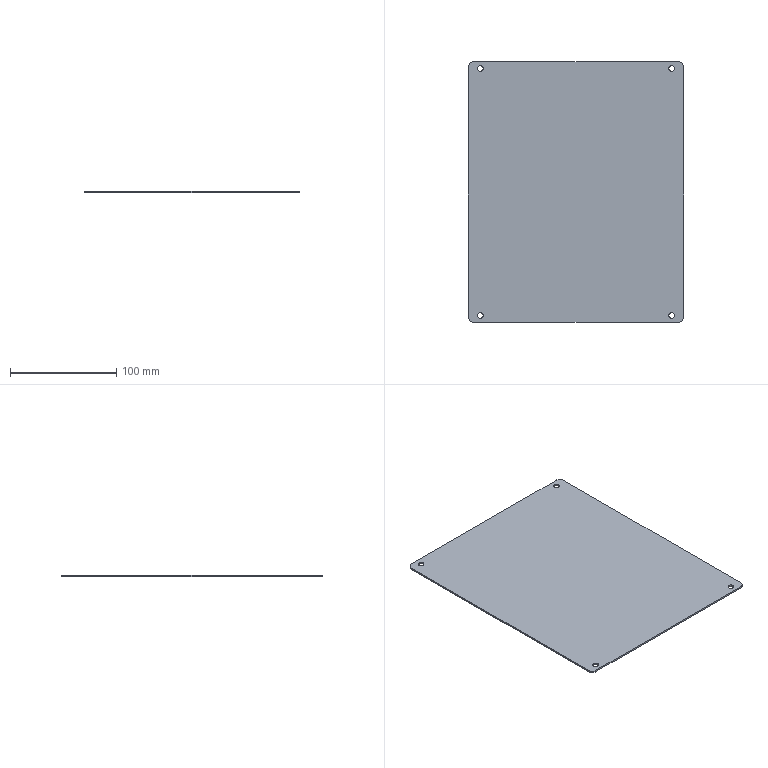Part | NX | features BREP 1 | 1 solid | 14 faces | box 202 x 245 x 1.5 mm | volume 74060 mm3 | cylinder 8 | plane 6 | commonest cylinder face diameters 5.5 x4 10 x4
STEP:
#1=CARTESIAN_POINT('',(-92.75,116.,0.));
#2=VERTEX_POINT('',#1);
#3=CARTESIAN_POINT('',(-90.,116.,0.));
#4=DIRECTION('',(0.,0.,1.));
#5=DIRECTION('',(-1.,0.,0.));
#6=AXIS2_PLACEMENT_3D('',#3,#4,#5);
#7=CIRCLE('',#6,2.75);
#8=EDGE_CURVE('',#2,#2,#7,.T.);
#9=ORIENTED_EDGE('',*,*,#8,.T.);
#10=EDGE_LOOP('',(#9));
#11=FACE_BOUND('',#10,.T.);
#12=CARTESIAN_POINT('',(-92.75,116.,-1.5));
#13=VERTEX_POINT('',#12);
#14=CARTESIAN_POINT('',(-90.,116.,-1.5));
#15=DIRECTION('',(0.,0.,-1.));
#16=DIRECTION('',(-1.,0.,0.));
#17=AXIS2_PLACEMENT_3D('',#14,#15,#16);
#18=CIRCLE('',#17,2.75);
#19=EDGE_CURVE('',#13,#13,#18,.T.);
#20=ORIENTED_EDGE('',*,*,#19,.T.);
#21=EDGE_LOOP('',(#20));
#22=FACE_BOUND('',#21,.T.);
#23=CARTESIAN_POINT('',(-90.,116.,-10.));
#24=DIRECTION('',(0.,0.,1.));
#25=DIRECTION('',(1.,0.,0.));
#26=AXIS2_PLACEMENT_3D('',#23,#24,#25);
#27=CYLINDRICAL_SURFACE('',#26,2.75);
#28=ADVANCED_FACE('',(#11,#22),#27,.F.);
#29=CARTESIAN_POINT('',(87.25,116.,0.));
#30=VERTEX_POINT('',#29);
#31=CARTESIAN_POINT('',(90.,116.,0.));
#32=DIRECTION('',(0.,0.,1.));
#33=DIRECTION('',(-1.,0.,0.));
#34=AXIS2_PLACEMENT_3D('',#31,#32,#33);
#35=CIRCLE('',#34,2.75);
#36=EDGE_CURVE('',#30,#30,#35,.T.);
#37=ORIENTED_EDGE('',*,*,#36,.T.);
#38=EDGE_LOOP('',(#37));
#39=FACE_BOUND('',#38,.T.);
#40=CARTESIAN_POINT('',(87.25,116.,-1.5));
#41=VERTEX_POINT('',#40);
#42=CARTESIAN_POINT('',(90.,116.,-1.5));
#43=DIRECTION('',(0.,0.,-1.));
#44=DIRECTION('',(-1.,0.,0.));
#45=AXIS2_PLACEMENT_3D('',#42,#43,#44);
#46=CIRCLE('',#45,2.75);
#47=EDGE_CURVE('',#41,#41,#46,.T.);
#48=ORIENTED_EDGE('',*,*,#47,.T.);
#49=EDGE_LOOP('',(#48));
#50=FACE_BOUND('',#49,.T.);
#51=CARTESIAN_POINT('',(90.,116.,-10.));
#52=DIRECTION('',(0.,0.,1.));
#53=DIRECTION('',(1.,0.,0.));
#54=AXIS2_PLACEMENT_3D('',#51,#52,#53);
#55=CYLINDRICAL_SURFACE('',#54,2.75);
#56=ADVANCED_FACE('',(#39,#50),#55,.F.);
#57=CARTESIAN_POINT('',(92.75,-116.,0.));
#58=VERTEX_POINT('',#57);
#59=CARTESIAN_POINT('',(90.,-116.,0.));
#60=DIRECTION('',(0.,0.,1.));
#61=DIRECTION('',(1.,0.,0.));
#62=AXIS2_PLACEMENT_3D('',#59,#60,#61);
#63=CIRCLE('',#62,2.75);
#64=EDGE_CURVE('',#58,#58,#63,.T.);
#65=ORIENTED_EDGE('',*,*,#64,.T.);
#66=EDGE_LOOP('',(#65));
#67=FACE_BOUND('',#66,.T.);
#68=CARTESIAN_POINT('',(87.25,-116.,-1.5));
#69=VERTEX_POINT('',#68);
#70=CARTESIAN_POINT('',(90.,-116.,-1.5));
#71=DIRECTION('',(0.,0.,-1.));
#72=DIRECTION('',(-1.,0.,0.));
#73=AXIS2_PLACEMENT_3D('',#70,#71,#72);
#74=CIRCLE('',#73,2.75);
#75=EDGE_CURVE('',#69,#69,#74,.T.);
#76=ORIENTED_EDGE('',*,*,#75,.T.);
#77=EDGE_LOOP('',(#76));
#78=FACE_BOUND('',#77,.T.);
#79=CARTESIAN_POINT('',(90.,-116.,-10.));
#80=DIRECTION('',(0.,0.,1.));
#81=DIRECTION('',(1.,0.,0.));
#82=AXIS2_PLACEMENT_3D('',#79,#80,#81);
#83=CYLINDRICAL_SURFACE('',#82,2.75);
#84=ADVANCED_FACE('',(#67,#78),#83,.F.);
#85=CARTESIAN_POINT('',(-87.25,-116.,0.));
#86=VERTEX_POINT('',#85);
#87=CARTESIAN_POINT('',(-90.,-116.,0.));
#88=DIRECTION('',(0.,0.,1.));
#89=DIRECTION('',(1.,0.,0.));
#90=AXIS2_PLACEMENT_3D('',#87,#88,#89);
#91=CIRCLE('',#90,2.75);
#92=EDGE_CURVE('',#86,#86,#91,.T.);
#93=ORIENTED_EDGE('',*,*,#92,.T.);
#94=EDGE_LOOP('',(#93));
#95=FACE_BOUND('',#94,.T.);
#96=CARTESIAN_POINT('',(-92.75,-116.,-1.5));
#97=VERTEX_POINT('',#96);
#98=CARTESIAN_POINT('',(-90.,-116.,-1.5));
#99=DIRECTION('',(0.,0.,-1.));
#100=DIRECTION('',(-1.,0.,0.));
#101=AXIS2_PLACEMENT_3D('',#98,#99,#100);
#102=CIRCLE('',#101,2.75);
#103=EDGE_CURVE('',#97,#97,#102,.T.);
#104=ORIENTED_EDGE('',*,*,#103,.T.);
#105=EDGE_LOOP('',(#104));
#106=FACE_BOUND('',#105,.T.);
#107=CARTESIAN_POINT('',(-90.,-116.,-10.));
#108=DIRECTION('',(0.,0.,1.));
#109=DIRECTION('',(1.,0.,0.));
#110=AXIS2_PLACEMENT_3D('',#107,#108,#109);
#111=CYLINDRICAL_SURFACE('',#110,2.75);
#112=ADVANCED_FACE('',(#95,#106),#111,.F.);
#113=CARTESIAN_POINT('',(101.,-117.5,0.));
#114=VERTEX_POINT('',#113);
#115=CARTESIAN_POINT('',(101.,117.5,0.));
#116=VERTEX_POINT('',#115);
#117=CARTESIAN_POINT('',(101.,-122.5,0.));
#118=DIRECTION('',(0.,1.,0.));
#119=VECTOR('',#118,1000.);
#120=LINE('',#117,#119);
#121=EDGE_CURVE('',#114,#116,#120,.T.);
#122=ORIENTED_EDGE('',*,*,#121,.F.);
#123=CARTESIAN_POINT('',(101.,-117.5,-1.5));
#124=VERTEX_POINT('',#123);
#125=CARTESIAN_POINT('',(101.,-117.5,-1.5));
#126=DIRECTION('',(0.,0.,-1.));
#127=VECTOR('',#126,1000.);
#128=LINE('',#125,#127);
#129=EDGE_CURVE('',#114,#124,#128,.T.);
#130=ORIENTED_EDGE('',*,*,#129,.T.);
#131=CARTESIAN_POINT('',(101.,117.5,-1.5));
#132=VERTEX_POINT('',#131);
#133=CARTESIAN_POINT('',(101.,-122.5,-1.5));
#134=DIRECTION('',(0.,1.,0.));
#135=VECTOR('',#134,1000.);
#136=LINE('',#133,#135);
#137=EDGE_CURVE('',#124,#132,#136,.T.);
#138=ORIENTED_EDGE('',*,*,#137,.T.);
#139=CARTESIAN_POINT('',(101.,117.5,-1.5));
#140=DIRECTION('',(0.,0.,1.));
#141=VECTOR('',#140,1000.);
#142=LINE('',#139,#141);
#143=EDGE_CURVE('',#132,#116,#142,.T.);
#144=ORIENTED_EDGE('',*,*,#143,.T.);
#145=EDGE_LOOP('',(#122,#130,#138,#144));
#146=FACE_BOUND('',#145,.T.);
#147=CARTESIAN_POINT('',(101.,-122.5,-1.5));
#148=DIRECTION('',(1.,0.,0.));
#149=DIRECTION('',(0.,0.,-1.));
#150=AXIS2_PLACEMENT_3D('',#147,#148,#149);
#151=PLANE('',#150);
#152=ADVANCED_FACE('',(#146),#151,.T.);
#153=CARTESIAN_POINT('',(-96.,-122.5,-1.5));
#154=VERTEX_POINT('',#153);
#155=CARTESIAN_POINT('',(96.,-122.5,-1.5));
#156=VERTEX_POINT('',#155);
#157=CARTESIAN_POINT('',(-101.,-122.5,-1.5));
#158=DIRECTION('',(1.,0.,0.));
#159=VECTOR('',#158,1000.);
#160=LINE('',#157,#159);
#161=EDGE_CURVE('',#154,#156,#160,.T.);
#162=ORIENTED_EDGE('',*,*,#161,.T.);
#163=CARTESIAN_POINT('',(96.,-122.5,0.));
#164=VERTEX_POINT('',#163);
#165=CARTESIAN_POINT('',(96.,-122.5,-1.5));
#166=DIRECTION('',(0.,0.,1.));
#167=VECTOR('',#166,1000.);
#168=LINE('',#165,#167);
#169=EDGE_CURVE('',#156,#164,#168,.T.);
#170=ORIENTED_EDGE('',*,*,#169,.T.);
#171=CARTESIAN_POINT('',(-96.,-122.5,0.));
#172=VERTEX_POINT('',#171);
#173=CARTESIAN_POINT('',(-101.,-122.5,0.));
#174=DIRECTION('',(1.,0.,0.));
#175=VECTOR('',#174,1000.);
#176=LINE('',#173,#175);
#177=EDGE_CURVE('',#172,#164,#176,.T.);
#178=ORIENTED_EDGE('',*,*,#177,.F.);
#179=CARTESIAN_POINT('',(-96.,-122.5,-1.5));
#180=DIRECTION('',(0.,0.,-1.));
#181=VECTOR('',#180,1000.);
#182=LINE('',#179,#181);
#183=EDGE_CURVE('',#172,#154,#182,.T.);
#184=ORIENTED_EDGE('',*,*,#183,.T.);
#185=EDGE_LOOP('',(#162,#170,#178,#184));
#186=FACE_BOUND('',#185,.T.);
#187=CARTESIAN_POINT('',(-101.,-122.5,-1.5));
#188=DIRECTION('',(0.,-1.,0.));
#189=DIRECTION('',(0.,0.,-1.));
#190=AXIS2_PLACEMENT_3D('',#187,#188,#189);
#191=PLANE('',#190);
#192=ADVANCED_FACE('',(#186),#191,.T.);
#193=CARTESIAN_POINT('',(-101.,117.5,0.));
#194=VERTEX_POINT('',#193);
#195=CARTESIAN_POINT('',(-101.,-117.5,0.));
#196=VERTEX_POINT('',#195);
#197=CARTESIAN_POINT('',(-101.,-122.5,0.));
#198=DIRECTION('',(0.,-1.,0.));
#199=VECTOR('',#198,1000.);
#200=LINE('',#197,#199);
#201=EDGE_CURVE('',#194,#196,#200,.T.);
#202=ORIENTED_EDGE('',*,*,#201,.F.);
#203=CARTESIAN_POINT('',(-101.,117.5,-1.5));
#204=VERTEX_POINT('',#203);
#205=CARTESIAN_POINT('',(-101.,117.5,-1.5));
#206=DIRECTION('',(0.,0.,-1.));
#207=VECTOR('',#206,1000.);
#208=LINE('',#205,#207);
#209=EDGE_CURVE('',#194,#204,#208,.T.);
#210=ORIENTED_EDGE('',*,*,#209,.T.);
#211=CARTESIAN_POINT('',(-101.,-117.5,-1.5));
#212=VERTEX_POINT('',#211);
#213=CARTESIAN_POINT('',(-101.,-122.5,-1.5));
#214=DIRECTION('',(0.,-1.,0.));
#215=VECTOR('',#214,1000.);
#216=LINE('',#213,#215);
#217=EDGE_CURVE('',#204,#212,#216,.T.);
#218=ORIENTED_EDGE('',*,*,#217,.T.);
#219=CARTESIAN_POINT('',(-101.,-117.5,-1.5));
#220=DIRECTION('',(0.,0.,1.));
#221=VECTOR('',#220,1000.);
#222=LINE('',#219,#221);
#223=EDGE_CURVE('',#212,#196,#222,.T.);
#224=ORIENTED_EDGE('',*,*,#223,.T.);
#225=EDGE_LOOP('',(#202,#210,#218,#224));
#226=FACE_BOUND('',#225,.T.);
#227=CARTESIAN_POINT('',(-101.,-122.5,-1.5));
#228=DIRECTION('',(-1.,0.,0.));
#229=DIRECTION('',(0.,0.,1.));
#230=AXIS2_PLACEMENT_3D('',#227,#228,#229);
#231=PLANE('',#230);
#232=ADVANCED_FACE('',(#226),#231,.T.);
#233=CARTESIAN_POINT('',(96.,122.5,0.));
#234=VERTEX_POINT('',#233);
#235=CARTESIAN_POINT('',(-96.,122.5,0.));
#236=VERTEX_POINT('',#235);
#237=CARTESIAN_POINT('',(-101.,122.5,0.));
#238=DIRECTION('',(-1.,0.,0.));
#239=VECTOR('',#238,1000.);
#240=LINE('',#237,#239);
#241=EDGE_CURVE('',#234,#236,#240,.T.);
#242=ORIENTED_EDGE('',*,*,#241,.F.);
#243=CARTESIAN_POINT('',(96.,122.5,-1.5));
#244=VERTEX_POINT('',#243);
#245=CARTESIAN_POINT('',(96.,122.5,-1.5));
#246=DIRECTION('',(0.,0.,-1.));
#247=VECTOR('',#246,1000.);
#248=LINE('',#245,#247);
#249=EDGE_CURVE('',#234,#244,#248,.T.);
#250=ORIENTED_EDGE('',*,*,#249,.T.);
#251=CARTESIAN_POINT('',(-96.,122.5,-1.5));
#252=VERTEX_POINT('',#251);
#253=CARTESIAN_POINT('',(-101.,122.5,-1.5));
#254=DIRECTION('',(-1.,0.,0.));
#255=VECTOR('',#254,1000.);
#256=LINE('',#253,#255);
#257=EDGE_CURVE('',#244,#252,#256,.T.);
#258=ORIENTED_EDGE('',*,*,#257,.T.);
#259=CARTESIAN_POINT('',(-96.,122.5,-1.5));
#260=DIRECTION('',(0.,0.,1.));
#261=VECTOR('',#260,1000.);
#262=LINE('',#259,#261);
#263=EDGE_CURVE('',#252,#236,#262,.T.);
#264=ORIENTED_EDGE('',*,*,#263,.T.);
#265=EDGE_LOOP('',(#242,#250,#258,#264));
#266=FACE_BOUND('',#265,.T.);
#267=CARTESIAN_POINT('',(-101.,122.5,-1.5));
#268=DIRECTION('',(0.,1.,0.));
#269=DIRECTION('',(0.,0.,1.));
#270=AXIS2_PLACEMENT_3D('',#267,#268,#269);
#271=PLANE('',#270);
#272=ADVANCED_FACE('',(#266),#271,.T.);
#273=ORIENTED_EDGE('',*,*,#19,.F.);
#274=EDGE_LOOP('',(#273));
#275=FACE_BOUND('',#274,.T.);
#276=ORIENTED_EDGE('',*,*,#47,.F.);
#277=EDGE_LOOP('',(#276));
#278=FACE_BOUND('',#277,.T.);
#279=ORIENTED_EDGE('',*,*,#75,.F.);
#280=EDGE_LOOP('',(#279));
#281=FACE_BOUND('',#280,.T.);
#282=ORIENTED_EDGE('',*,*,#103,.F.);
#283=EDGE_LOOP('',(#282));
#284=FACE_BOUND('',#283,.T.);
#285=ORIENTED_EDGE('',*,*,#137,.F.);
#286=CARTESIAN_POINT('',(96.,-117.5,-1.5));
#287=DIRECTION('',(0.,0.,-1.));
#288=DIRECTION('',(-1.,0.,0.));
#289=AXIS2_PLACEMENT_3D('',#286,#287,#288);
#290=CIRCLE('',#289,5.);
#291=EDGE_CURVE('',#124,#156,#290,.T.);
#292=ORIENTED_EDGE('',*,*,#291,.T.);
#293=ORIENTED_EDGE('',*,*,#161,.F.);
#294=CARTESIAN_POINT('',(-96.,-117.5,-1.5));
#295=DIRECTION('',(0.,0.,-1.));
#296=DIRECTION('',(-1.,0.,0.));
#297=AXIS2_PLACEMENT_3D('',#294,#295,#296);
#298=CIRCLE('',#297,5.);
#299=EDGE_CURVE('',#154,#212,#298,.T.);
#300=ORIENTED_EDGE('',*,*,#299,.T.);
#301=ORIENTED_EDGE('',*,*,#217,.F.);
#302=CARTESIAN_POINT('',(-96.,117.5,-1.5));
#303=DIRECTION('',(0.,0.,-1.));
#304=DIRECTION('',(-1.,0.,0.));
#305=AXIS2_PLACEMENT_3D('',#302,#303,#304);
#306=CIRCLE('',#305,5.);
#307=EDGE_CURVE('',#204,#252,#306,.T.);
#308=ORIENTED_EDGE('',*,*,#307,.T.);
#309=ORIENTED_EDGE('',*,*,#257,.F.);
#310=CARTESIAN_POINT('',(96.,117.5,-1.5));
#311=DIRECTION('',(0.,0.,-1.));
#312=DIRECTION('',(-1.,0.,0.));
#313=AXIS2_PLACEMENT_3D('',#310,#311,#312);
#314=CIRCLE('',#313,5.);
#315=EDGE_CURVE('',#244,#132,#314,.T.);
#316=ORIENTED_EDGE('',*,*,#315,.T.);
#317=EDGE_LOOP('',(#285,#292,#293,#300,#301,#308,#309,#316));
#318=FACE_BOUND('',#317,.T.);
#319=CARTESIAN_POINT('',(0.,0.,-1.5));
#320=DIRECTION('',(0.,0.,-1.));
#321=DIRECTION('',(-1.,0.,0.));
#322=AXIS2_PLACEMENT_3D('',#319,#320,#321);
#323=PLANE('',#322);
#324=ADVANCED_FACE('',(#275,#278,#281,#284,#318),#323,.T.);
#325=ORIENTED_EDGE('',*,*,#8,.F.);
#326=EDGE_LOOP('',(#325));
#327=FACE_BOUND('',#326,.T.);
#328=ORIENTED_EDGE('',*,*,#36,.F.);
#329=EDGE_LOOP('',(#328));
#330=FACE_BOUND('',#329,.T.);
#331=ORIENTED_EDGE('',*,*,#64,.F.);
#332=EDGE_LOOP('',(#331));
#333=FACE_BOUND('',#332,.T.);
#334=ORIENTED_EDGE('',*,*,#92,.F.);
#335=EDGE_LOOP('',(#334));
#336=FACE_BOUND('',#335,.T.);
#337=ORIENTED_EDGE('',*,*,#177,.T.);
#338=CARTESIAN_POINT('',(96.,-117.5,0.));
#339=DIRECTION('',(0.,0.,1.));
#340=DIRECTION('',(-1.,0.,0.));
#341=AXIS2_PLACEMENT_3D('',#338,#339,#340);
#342=CIRCLE('',#341,5.);
#343=EDGE_CURVE('',#164,#114,#342,.T.);
#344=ORIENTED_EDGE('',*,*,#343,.T.);
#345=ORIENTED_EDGE('',*,*,#121,.T.);
#346=CARTESIAN_POINT('',(96.,117.5,0.));
#347=DIRECTION('',(0.,0.,1.));
#348=DIRECTION('',(-1.,0.,0.));
#349=AXIS2_PLACEMENT_3D('',#346,#347,#348);
#350=CIRCLE('',#349,5.);
#351=EDGE_CURVE('',#116,#234,#350,.T.);
#352=ORIENTED_EDGE('',*,*,#351,.T.);
#353=ORIENTED_EDGE('',*,*,#241,.T.);
#354=CARTESIAN_POINT('',(-96.,117.5,0.));
#355=DIRECTION('',(0.,0.,1.));
#356=DIRECTION('',(-1.,0.,0.));
#357=AXIS2_PLACEMENT_3D('',#354,#355,#356);
#358=CIRCLE('',#357,5.);
#359=EDGE_CURVE('',#236,#194,#358,.T.);
#360=ORIENTED_EDGE('',*,*,#359,.T.);
#361=ORIENTED_EDGE('',*,*,#201,.T.);
#362=CARTESIAN_POINT('',(-96.,-117.5,0.));
#363=DIRECTION('',(0.,0.,1.));
#364=DIRECTION('',(-1.,0.,0.));
#365=AXIS2_PLACEMENT_3D('',#362,#363,#364);
#366=CIRCLE('',#365,5.);
#367=EDGE_CURVE('',#196,#172,#366,.T.);
#368=ORIENTED_EDGE('',*,*,#367,.T.);
#369=EDGE_LOOP('',(#337,#344,#345,#352,#353,#360,#361,#368));
#370=FACE_BOUND('',#369,.T.);
#371=CARTESIAN_POINT('',(0.,0.,0.));
#372=DIRECTION('',(0.,0.,-1.));
#373=DIRECTION('',(-1.,0.,0.));
#374=AXIS2_PLACEMENT_3D('',#371,#372,#373);
#375=PLANE('',#374);
#376=ADVANCED_FACE('',(#327,#330,#333,#336,#370),#375,.F.);
#377=ORIENTED_EDGE('',*,*,#291,.F.);
#378=ORIENTED_EDGE('',*,*,#129,.F.);
#379=ORIENTED_EDGE('',*,*,#343,.F.);
#380=ORIENTED_EDGE('',*,*,#169,.F.);
#381=EDGE_LOOP('',(#377,#378,#379,#380));
#382=FACE_BOUND('',#381,.T.);
#383=CARTESIAN_POINT('',(96.,-117.5,-1.5));
#384=DIRECTION('',(0.,0.,1.));
#385=DIRECTION('',(1.,0.,0.));
#386=AXIS2_PLACEMENT_3D('',#383,#384,#385);
#387=CYLINDRICAL_SURFACE('',#386,5.);
#388=ADVANCED_FACE('',(#382),#387,.T.);
#389=ORIENTED_EDGE('',*,*,#315,.F.);
#390=ORIENTED_EDGE('',*,*,#249,.F.);
#391=ORIENTED_EDGE('',*,*,#351,.F.);
#392=ORIENTED_EDGE('',*,*,#143,.F.);
#393=EDGE_LOOP('',(#389,#390,#391,#392));
#394=FACE_BOUND('',#393,.T.);
#395=CARTESIAN_POINT('',(96.,117.5,-1.5));
#396=DIRECTION('',(0.,0.,1.));
#397=DIRECTION('',(1.,0.,0.));
#398=AXIS2_PLACEMENT_3D('',#395,#396,#397);
#399=CYLINDRICAL_SURFACE('',#398,5.);
#400=ADVANCED_FACE('',(#394),#399,.T.);
#401=ORIENTED_EDGE('',*,*,#307,.F.);
#402=ORIENTED_EDGE('',*,*,#209,.F.);
#403=ORIENTED_EDGE('',*,*,#359,.F.);
#404=ORIENTED_EDGE('',*,*,#263,.F.);
#405=EDGE_LOOP('',(#401,#402,#403,#404));
#406=FACE_BOUND('',#405,.T.);
#407=CARTESIAN_POINT('',(-96.,117.5,-1.5));
#408=DIRECTION('',(0.,0.,1.));
#409=DIRECTION('',(1.,0.,0.));
#410=AXIS2_PLACEMENT_3D('',#407,#408,#409);
#411=CYLINDRICAL_SURFACE('',#410,5.);
#412=ADVANCED_FACE('',(#406),#411,.T.);
#413=ORIENTED_EDGE('',*,*,#299,.F.);
#414=ORIENTED_EDGE('',*,*,#183,.F.);
#415=ORIENTED_EDGE('',*,*,#367,.F.);
#416=ORIENTED_EDGE('',*,*,#223,.F.);
#417=EDGE_LOOP('',(#413,#414,#415,#416));
#418=FACE_BOUND('',#417,.T.);
#419=CARTESIAN_POINT('',(-96.,-117.5,-1.5));
#420=DIRECTION('',(0.,0.,1.));
#421=DIRECTION('',(1.,0.,0.));
#422=AXIS2_PLACEMENT_3D('',#419,#420,#421);
#423=CYLINDRICAL_SURFACE('',#422,5.);
#424=ADVANCED_FACE('',(#418),#423,.T.);
#425=CLOSED_SHELL('',(#28,#56,#84,#112,#152,#192,#232,#272,#324,#376,#388,#400,#412,#424));
#426=MANIFOLD_SOLID_BREP('',#425);
#427=(LENGTH_UNIT()NAMED_UNIT(*)SI_UNIT(.MILLI.,.METRE.));
#428=UNCERTAINTY_MEASURE_WITH_UNIT(LENGTH_MEASURE(0.00001),#427,'','');
#429=(NAMED_UNIT(*)PLANE_ANGLE_UNIT()SI_UNIT($,.RADIAN.));
#430=(NAMED_UNIT(*)SI_UNIT($,.STERADIAN.)SOLID_ANGLE_UNIT());
#431=(GEOMETRIC_REPRESENTATION_CONTEXT(3)GLOBAL_UNCERTAINTY_ASSIGNED_CONTEXT((#428))GLOBAL_UNIT_ASSIGNED_CONTEXT((#427,#429,#430))REPRESENTATION_CONTEXT('',''));
#432=ADVANCED_BREP_SHAPE_REPRESENTATION('',(#426),#431);